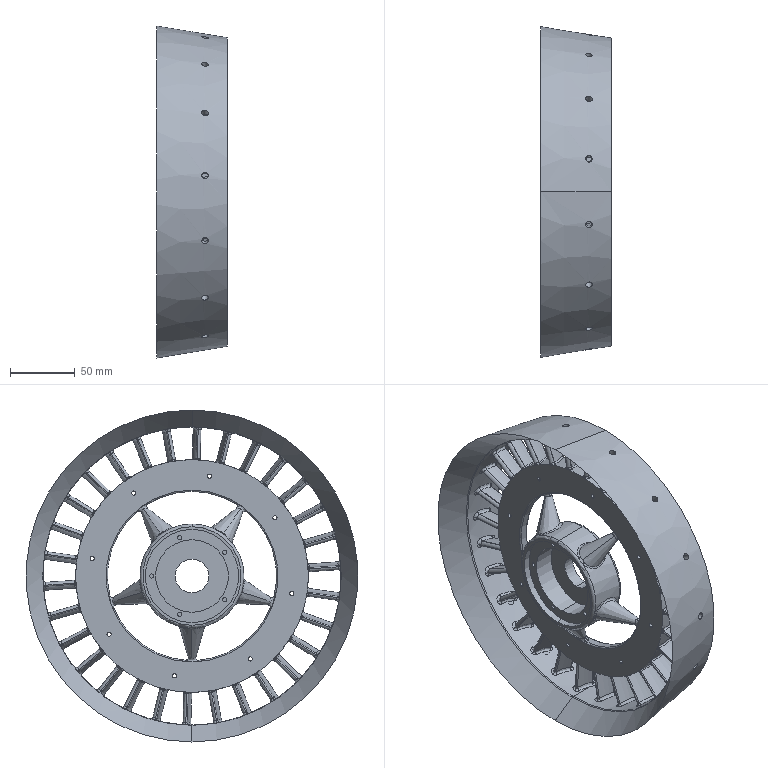Part | STEP file | Completa.sldasm-Part-23_Valor predeterminado | 1 solid | 937 faces | box 54.453 x 255.658 x 255.658 mm | volume 510804 mm3 | spline 480 | cylinder 318 | torus 87 | plane 28 | cone 14 | other 10 | commonest cylinder face diameters 1.234 x60 4.937 x60 178.959 x31 1.481 x30 5 x30 66.068 x30